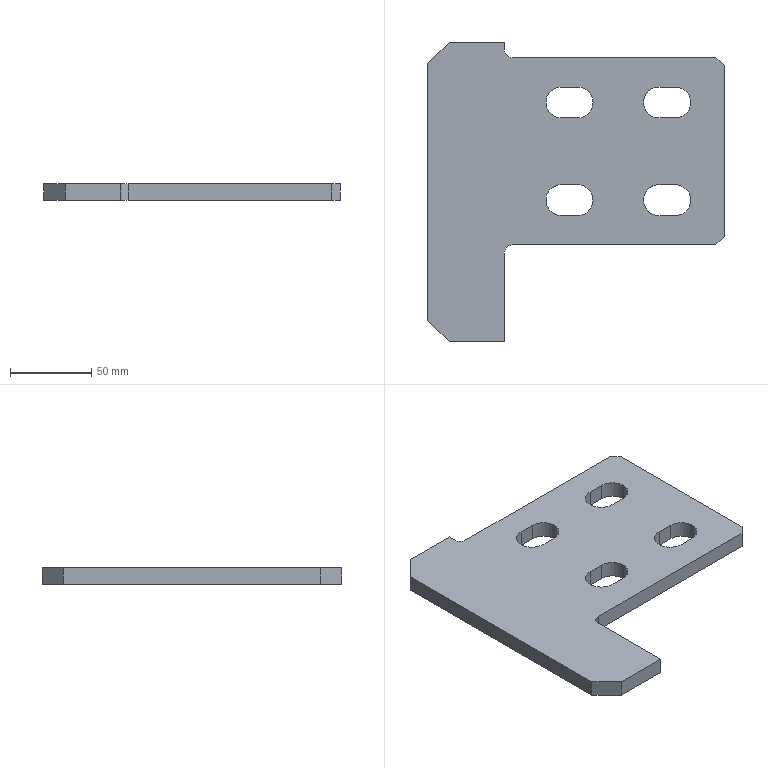Part | STEP file | 筋Plate-200×100-150 | 1 solid | 36 faces | box 182 x 184 x 10 mm | volume 220956 mm3 | plane 22 | cylinder 14 | commonest cylinder face diameters 19 x12 10 x2